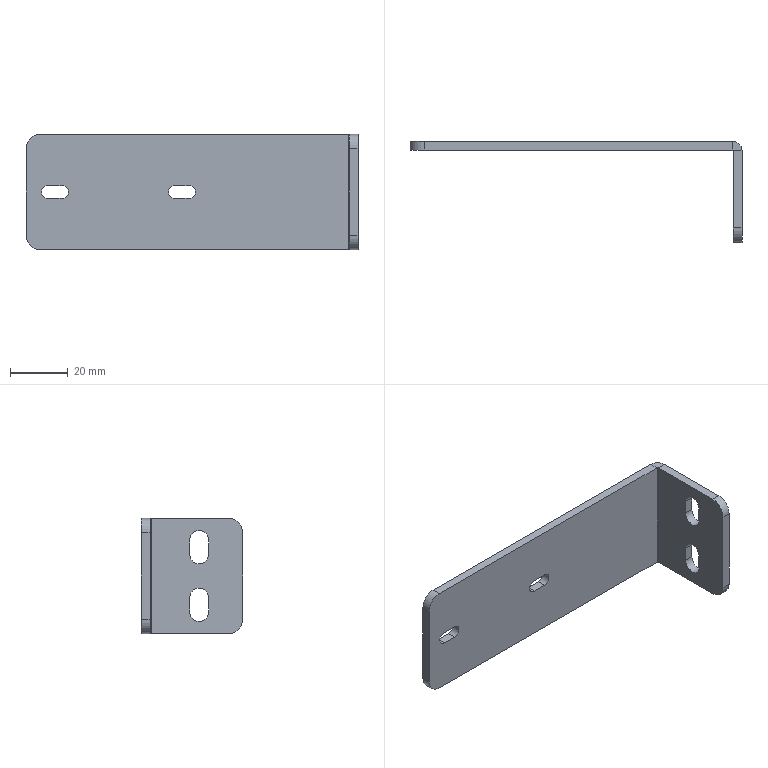Part | SolidWorks | features ICE 2, Fillet 1, FlatPattern 1, HoleWzd 1, SMBaseFlange 1, SheetMetal 1 | 1 solid | 34 faces | box 115 x 35 x 40 mm | volume 16866 mm3 | plane 20 | cylinder 14 | commonest cylinder face diameters 4.4 x4 6.5 x4 10 x4 0.6 x1 6.6 x1
STEP:
#1=CARTESIAN_POINT('',(115.,-3.3,40.));
#2=VERTEX_POINT('',#1);
#3=CARTESIAN_POINT('',(112.,-3.3,40.));
#4=VERTEX_POINT('',#3);
#5=CARTESIAN_POINT('',(115.,-3.3,40.));
#6=DIRECTION('',(-1.,0.,0.));
#7=VECTOR('',#6,1000.);
#8=LINE('',#5,#7);
#9=EDGE_CURVE('',#2,#4,#8,.T.);
#10=ORIENTED_EDGE('',*,*,#9,.F.);
#11=CARTESIAN_POINT('',(111.7,0.,40.));
#12=VERTEX_POINT('',#11);
#13=CARTESIAN_POINT('',(111.7,-3.3,40.));
#14=DIRECTION('',(0.,0.,-1.));
#15=DIRECTION('',(1.,0.,0.));
#16=AXIS2_PLACEMENT_3D('',#13,#14,#15);
#17=CIRCLE('',#16,3.3);
#18=EDGE_CURVE('',#12,#2,#17,.T.);
#19=ORIENTED_EDGE('',*,*,#18,.F.);
#20=CARTESIAN_POINT('',(111.7,-3.,40.));
#21=VERTEX_POINT('',#20);
#22=CARTESIAN_POINT('',(111.7,-3.,40.));
#23=DIRECTION('',(0.,1.,0.));
#24=VECTOR('',#23,1000.);
#25=LINE('',#22,#24);
#26=EDGE_CURVE('',#21,#12,#25,.T.);
#27=ORIENTED_EDGE('',*,*,#26,.F.);
#28=CARTESIAN_POINT('',(111.7,-3.3,40.));
#29=DIRECTION('',(0.,0.,-1.));
#30=DIRECTION('',(1.,0.,0.));
#31=AXIS2_PLACEMENT_3D('',#28,#29,#30);
#32=CIRCLE('',#31,0.3);
#33=EDGE_CURVE('',#21,#4,#32,.T.);
#34=ORIENTED_EDGE('',*,*,#33,.T.);
#35=EDGE_LOOP('',(#10,#19,#27,#34));
#36=FACE_OUTER_BOUND('',#35,.T.);
#37=CARTESIAN_POINT('',(115.,-3.3,40.));
#38=DIRECTION('',(0.,0.,1.));
#39=DIRECTION('',(1.,0.,0.));
#40=AXIS2_PLACEMENT_3D('',#37,#38,#39);
#41=PLANE('',#40);
#42=ADVANCED_FACE('',(#36),#41,.T.);
#43=CARTESIAN_POINT('',(112.,-30.,40.));
#44=VERTEX_POINT('',#43);
#45=CARTESIAN_POINT('',(112.,0.,40.));
#46=DIRECTION('',(0.,-1.,0.));
#47=VECTOR('',#46,1000.);
#48=LINE('',#45,#47);
#49=EDGE_CURVE('',#4,#44,#48,.T.);
#50=ORIENTED_EDGE('',*,*,#49,.T.);
#51=CARTESIAN_POINT('',(115.,-30.,40.));
#52=VERTEX_POINT('',#51);
#53=CARTESIAN_POINT('',(111.7,-30.,40.));
#54=DIRECTION('',(1.,0.,0.));
#55=VECTOR('',#54,1000.);
#56=LINE('',#53,#55);
#57=EDGE_CURVE('',#44,#52,#56,.T.);
#58=ORIENTED_EDGE('',*,*,#57,.T.);
#59=CARTESIAN_POINT('',(115.,0.,40.));
#60=DIRECTION('',(0.,-1.,0.));
#61=VECTOR('',#60,1000.);
#62=LINE('',#59,#61);
#63=EDGE_CURVE('',#2,#52,#62,.T.);
#64=ORIENTED_EDGE('',*,*,#63,.F.);
#65=ORIENTED_EDGE('',*,*,#9,.T.);
#66=EDGE_LOOP('',(#50,#58,#64,#65));
#67=FACE_OUTER_BOUND('',#66,.T.);
#68=CARTESIAN_POINT('',(111.7,-3.,40.));
#69=DIRECTION('',(0.,0.,1.));
#70=DIRECTION('',(1.,0.,0.));
#71=AXIS2_PLACEMENT_3D('',#68,#69,#70);
#72=PLANE('',#71);
#73=ADVANCED_FACE('',(#67),#72,.T.);
#74=CARTESIAN_POINT('',(111.7,0.,0.));
#75=VERTEX_POINT('',#74);
#76=CARTESIAN_POINT('',(111.7,-3.,0.));
#77=VERTEX_POINT('',#76);
#78=CARTESIAN_POINT('',(111.7,0.,0.));
#79=DIRECTION('',(0.,-1.,0.));
#80=VECTOR('',#79,1000.);
#81=LINE('',#78,#80);
#82=EDGE_CURVE('',#75,#77,#81,.T.);
#83=ORIENTED_EDGE('',*,*,#82,.F.);
#84=CARTESIAN_POINT('',(115.,-3.3,0.));
#85=VERTEX_POINT('',#84);
#86=CARTESIAN_POINT('',(111.7,-3.3,0.));
#87=DIRECTION('',(0.,0.,-1.));
#88=DIRECTION('',(1.,0.,0.));
#89=AXIS2_PLACEMENT_3D('',#86,#87,#88);
#90=CIRCLE('',#89,3.3);
#91=EDGE_CURVE('',#75,#85,#90,.T.);
#92=ORIENTED_EDGE('',*,*,#91,.T.);
#93=CARTESIAN_POINT('',(112.,-3.3,0.));
#94=VERTEX_POINT('',#93);
#95=CARTESIAN_POINT('',(112.,-3.3,0.));
#96=DIRECTION('',(1.,0.,0.));
#97=VECTOR('',#96,1000.);
#98=LINE('',#95,#97);
#99=EDGE_CURVE('',#94,#85,#98,.T.);
#100=ORIENTED_EDGE('',*,*,#99,.F.);
#101=CARTESIAN_POINT('',(111.7,-3.3,0.));
#102=DIRECTION('',(0.,0.,-1.));
#103=DIRECTION('',(1.,0.,0.));
#104=AXIS2_PLACEMENT_3D('',#101,#102,#103);
#105=CIRCLE('',#104,0.3);
#106=EDGE_CURVE('',#77,#94,#105,.T.);
#107=ORIENTED_EDGE('',*,*,#106,.F.);
#108=EDGE_LOOP('',(#83,#92,#100,#107));
#109=FACE_OUTER_BOUND('',#108,.T.);
#110=CARTESIAN_POINT('',(111.7,0.,0.));
#111=DIRECTION('',(0.,0.,-1.));
#112=DIRECTION('',(-1.,0.,0.));
#113=AXIS2_PLACEMENT_3D('',#110,#111,#112);
#114=PLANE('',#113);
#115=ADVANCED_FACE('',(#109),#114,.T.);
#116=CARTESIAN_POINT('',(5.,-3.,0.));
#117=VERTEX_POINT('',#116);
#118=CARTESIAN_POINT('',(0.,-3.,0.));
#119=DIRECTION('',(1.,0.,0.));
#120=VECTOR('',#119,1000.);
#121=LINE('',#118,#120);
#122=EDGE_CURVE('',#117,#77,#121,.T.);
#123=ORIENTED_EDGE('',*,*,#122,.F.);
#124=CARTESIAN_POINT('',(5.,0.,0.));
#125=VERTEX_POINT('',#124);
#126=CARTESIAN_POINT('',(5.,-3.3,0.));
#127=DIRECTION('',(0.,1.,0.));
#128=VECTOR('',#127,1000.);
#129=LINE('',#126,#128);
#130=EDGE_CURVE('',#117,#125,#129,.T.);
#131=ORIENTED_EDGE('',*,*,#130,.T.);
#132=CARTESIAN_POINT('',(0.,0.,0.));
#133=DIRECTION('',(1.,0.,0.));
#134=VECTOR('',#133,1000.);
#135=LINE('',#132,#134);
#136=EDGE_CURVE('',#125,#75,#135,.T.);
#137=ORIENTED_EDGE('',*,*,#136,.T.);
#138=ORIENTED_EDGE('',*,*,#82,.T.);
#139=EDGE_LOOP('',(#123,#131,#137,#138));
#140=FACE_OUTER_BOUND('',#139,.T.);
#141=CARTESIAN_POINT('',(112.,-3.3,0.));
#142=DIRECTION('',(0.,0.,-1.));
#143=DIRECTION('',(-1.,0.,0.));
#144=AXIS2_PLACEMENT_3D('',#141,#142,#143);
#145=PLANE('',#144);
#146=ADVANCED_FACE('',(#140),#145,.T.);
#147=CARTESIAN_POINT('',(112.,-23.25,7.5));
#148=VERTEX_POINT('',#147);
#149=CARTESIAN_POINT('',(112.,-23.25,12.5));
#150=VERTEX_POINT('',#149);
#151=CARTESIAN_POINT('',(112.,-23.25,7.5));
#152=DIRECTION('',(0.,0.,1.));
#153=VECTOR('',#152,1000.);
#154=LINE('',#151,#153);
#155=EDGE_CURVE('',#148,#150,#154,.T.);
#156=ORIENTED_EDGE('',*,*,#155,.F.);
#157=CARTESIAN_POINT('',(112.,-16.75,7.5));
#158=VERTEX_POINT('',#157);
#159=CARTESIAN_POINT('',(112.,-20.,7.5));
#160=DIRECTION('',(-1.,0.,0.));
#161=DIRECTION('',(0.,-1.,0.));
#162=AXIS2_PLACEMENT_3D('',#159,#160,#161);
#163=CIRCLE('',#162,3.25);
#164=EDGE_CURVE('',#158,#148,#163,.T.);
#165=ORIENTED_EDGE('',*,*,#164,.F.);
#166=CARTESIAN_POINT('',(112.,-16.75,12.5));
#167=VERTEX_POINT('',#166);
#168=CARTESIAN_POINT('',(112.,-16.75,7.5));
#169=DIRECTION('',(0.,0.,-1.));
#170=VECTOR('',#169,1000.);
#171=LINE('',#168,#170);
#172=EDGE_CURVE('',#167,#158,#171,.T.);
#173=ORIENTED_EDGE('',*,*,#172,.F.);
#174=CARTESIAN_POINT('',(112.,-20.,12.5));
#175=DIRECTION('',(-1.,0.,0.));
#176=DIRECTION('',(0.,-1.,0.));
#177=AXIS2_PLACEMENT_3D('',#174,#175,#176);
#178=CIRCLE('',#177,3.25);
#179=EDGE_CURVE('',#150,#167,#178,.T.);
#180=ORIENTED_EDGE('',*,*,#179,.F.);
#181=EDGE_LOOP('',(#156,#165,#173,#180));
#182=FACE_BOUND('',#181,.T.);
#183=CARTESIAN_POINT('',(112.,-23.25,27.5));
#184=VERTEX_POINT('',#183);
#185=CARTESIAN_POINT('',(112.,-23.25,32.5));
#186=VERTEX_POINT('',#185);
#187=CARTESIAN_POINT('',(112.,-23.25,27.5));
#188=DIRECTION('',(0.,0.,1.));
#189=VECTOR('',#188,1000.);
#190=LINE('',#187,#189);
#191=EDGE_CURVE('',#184,#186,#190,.T.);
#192=ORIENTED_EDGE('',*,*,#191,.F.);
#193=CARTESIAN_POINT('',(112.,-16.75,27.5));
#194=VERTEX_POINT('',#193);
#195=CARTESIAN_POINT('',(112.,-20.,27.5));
#196=DIRECTION('',(-1.,0.,0.));
#197=DIRECTION('',(0.,-1.,0.));
#198=AXIS2_PLACEMENT_3D('',#195,#196,#197);
#199=CIRCLE('',#198,3.25);
#200=EDGE_CURVE('',#194,#184,#199,.T.);
#201=ORIENTED_EDGE('',*,*,#200,.F.);
#202=CARTESIAN_POINT('',(112.,-16.75,32.5));
#203=VERTEX_POINT('',#202);
#204=CARTESIAN_POINT('',(112.,-16.75,27.5));
#205=DIRECTION('',(0.,0.,-1.));
#206=VECTOR('',#205,1000.);
#207=LINE('',#204,#206);
#208=EDGE_CURVE('',#203,#194,#207,.T.);
#209=ORIENTED_EDGE('',*,*,#208,.F.);
#210=CARTESIAN_POINT('',(112.,-20.,32.5));
#211=DIRECTION('',(-1.,0.,0.));
#212=DIRECTION('',(0.,-1.,0.));
#213=AXIS2_PLACEMENT_3D('',#210,#211,#212);
#214=CIRCLE('',#213,3.25);
#215=EDGE_CURVE('',#186,#203,#214,.T.);
#216=ORIENTED_EDGE('',*,*,#215,.F.);
#217=EDGE_LOOP('',(#192,#201,#209,#216));
#218=FACE_BOUND('',#217,.T.);
#219=CARTESIAN_POINT('',(112.,-30.,0.));
#220=VERTEX_POINT('',#219);
#221=CARTESIAN_POINT('',(112.,0.,0.));
#222=DIRECTION('',(0.,-1.,0.));
#223=VECTOR('',#222,1000.);
#224=LINE('',#221,#223);
#225=EDGE_CURVE('',#94,#220,#224,.T.);
#226=ORIENTED_EDGE('',*,*,#225,.T.);
#227=CARTESIAN_POINT('',(112.,-35.,5.));
#228=VERTEX_POINT('',#227);
#229=CARTESIAN_POINT('',(112.,-30.,5.));
#230=DIRECTION('',(-1.,0.,0.));
#231=DIRECTION('',(0.,1.,0.));
#232=AXIS2_PLACEMENT_3D('',#229,#230,#231);
#233=CIRCLE('',#232,5.);
#234=EDGE_CURVE('',#220,#228,#233,.T.);
#235=ORIENTED_EDGE('',*,*,#234,.T.);
#236=CARTESIAN_POINT('',(112.,-35.,35.));
#237=VERTEX_POINT('',#236);
#238=CARTESIAN_POINT('',(112.,-35.,40.));
#239=DIRECTION('',(0.,0.,-1.));
#240=VECTOR('',#239,1000.);
#241=LINE('',#238,#240);
#242=EDGE_CURVE('',#237,#228,#241,.T.);
#243=ORIENTED_EDGE('',*,*,#242,.F.);
#244=CARTESIAN_POINT('',(112.,-30.,35.));
#245=DIRECTION('',(-1.,0.,0.));
#246=DIRECTION('',(0.,1.,0.));
#247=AXIS2_PLACEMENT_3D('',#244,#245,#246);
#248=CIRCLE('',#247,5.);
#249=EDGE_CURVE('',#237,#44,#248,.T.);
#250=ORIENTED_EDGE('',*,*,#249,.T.);
#251=ORIENTED_EDGE('',*,*,#49,.F.);
#252=CARTESIAN_POINT('',(112.,-3.3,40.));
#253=DIRECTION('',(0.,0.,-1.));
#254=VECTOR('',#253,1000.);
#255=LINE('',#252,#254);
#256=EDGE_CURVE('',#4,#94,#255,.T.);
#257=ORIENTED_EDGE('',*,*,#256,.T.);
#258=EDGE_LOOP('',(#226,#235,#243,#250,#251,#257));
#259=FACE_OUTER_BOUND('',#258,.T.);
#260=CARTESIAN_POINT('',(112.,0.,40.));
#261=DIRECTION('',(1.,0.,0.));
#262=DIRECTION('',(0.,1.,0.));
#263=AXIS2_PLACEMENT_3D('',#260,#261,#262);
#264=PLANE('',#263);
#265=ADVANCED_FACE('',(#182,#218,#259),#264,.F.);
#266=ORIENTED_EDGE('',*,*,#242,.T.);
#267=CARTESIAN_POINT('',(115.,-35.,5.));
#268=VERTEX_POINT('',#267);
#269=CARTESIAN_POINT('',(115.,-35.,5.));
#270=DIRECTION('',(1.,0.,0.));
#271=VECTOR('',#270,1000.);
#272=LINE('',#269,#271);
#273=EDGE_CURVE('',#228,#268,#272,.T.);
#274=ORIENTED_EDGE('',*,*,#273,.T.);
#275=CARTESIAN_POINT('',(115.,-35.,35.));
#276=VERTEX_POINT('',#275);
#277=CARTESIAN_POINT('',(115.,-35.,40.));
#278=DIRECTION('',(0.,0.,-1.));
#279=VECTOR('',#278,1000.);
#280=LINE('',#277,#279);
#281=EDGE_CURVE('',#276,#268,#280,.T.);
#282=ORIENTED_EDGE('',*,*,#281,.F.);
#283=CARTESIAN_POINT('',(115.,-35.,35.));
#284=DIRECTION('',(-1.,0.,0.));
#285=VECTOR('',#284,1000.);
#286=LINE('',#283,#285);
#287=EDGE_CURVE('',#276,#237,#286,.T.);
#288=ORIENTED_EDGE('',*,*,#287,.T.);
#289=EDGE_LOOP('',(#266,#274,#282,#288));
#290=FACE_OUTER_BOUND('',#289,.T.);
#291=CARTESIAN_POINT('',(115.,-35.,40.));
#292=DIRECTION('',(0.,-1.,0.));
#293=DIRECTION('',(0.,0.,-1.));
#294=AXIS2_PLACEMENT_3D('',#291,#292,#293);
#295=PLANE('',#294);
#296=ADVANCED_FACE('',(#290),#295,.T.);
#297=CARTESIAN_POINT('',(115.,-23.25,7.5));
#298=VERTEX_POINT('',#297);
#299=CARTESIAN_POINT('',(115.,-16.75,7.5));
#300=VERTEX_POINT('',#299);
#301=CARTESIAN_POINT('',(115.,-20.,7.5));
#302=DIRECTION('',(1.,0.,0.));
#303=DIRECTION('',(0.,1.,0.));
#304=AXIS2_PLACEMENT_3D('',#301,#302,#303);
#305=CIRCLE('',#304,3.25);
#306=EDGE_CURVE('',#298,#300,#305,.T.);
#307=ORIENTED_EDGE('',*,*,#306,.F.);
#308=CARTESIAN_POINT('',(115.,-23.25,12.5));
#309=VERTEX_POINT('',#308);
#310=CARTESIAN_POINT('',(115.,-23.25,40.));
#311=DIRECTION('',(0.,0.,-1.));
#312=VECTOR('',#311,1000.);
#313=LINE('',#310,#312);
#314=EDGE_CURVE('',#309,#298,#313,.T.);
#315=ORIENTED_EDGE('',*,*,#314,.F.);
#316=CARTESIAN_POINT('',(115.,-16.75,12.5));
#317=VERTEX_POINT('',#316);
#318=CARTESIAN_POINT('',(115.,-20.,12.5));
#319=DIRECTION('',(1.,0.,0.));
#320=DIRECTION('',(0.,1.,0.));
#321=AXIS2_PLACEMENT_3D('',#318,#319,#320);
#322=CIRCLE('',#321,3.25);
#323=EDGE_CURVE('',#317,#309,#322,.T.);
#324=ORIENTED_EDGE('',*,*,#323,.F.);
#325=CARTESIAN_POINT('',(115.,-16.75,40.));
#326=DIRECTION('',(0.,0.,1.));
#327=VECTOR('',#326,1000.);
#328=LINE('',#325,#327);
#329=EDGE_CURVE('',#300,#317,#328,.T.);
#330=ORIENTED_EDGE('',*,*,#329,.F.);
#331=EDGE_LOOP('',(#307,#315,#324,#330));
#332=FACE_BOUND('',#331,.T.);
#333=CARTESIAN_POINT('',(115.,-23.25,27.5));
#334=VERTEX_POINT('',#333);
#335=CARTESIAN_POINT('',(115.,-16.75,27.5));
#336=VERTEX_POINT('',#335);
#337=CARTESIAN_POINT('',(115.,-20.,27.5));
#338=DIRECTION('',(1.,0.,0.));
#339=DIRECTION('',(0.,1.,0.));
#340=AXIS2_PLACEMENT_3D('',#337,#338,#339);
#341=CIRCLE('',#340,3.25);
#342=EDGE_CURVE('',#334,#336,#341,.T.);
#343=ORIENTED_EDGE('',*,*,#342,.F.);
#344=CARTESIAN_POINT('',(115.,-23.25,32.5));
#345=VERTEX_POINT('',#344);
#346=CARTESIAN_POINT('',(115.,-23.25,40.));
#347=DIRECTION('',(0.,0.,-1.));
#348=VECTOR('',#347,1000.);
#349=LINE('',#346,#348);
#350=EDGE_CURVE('',#345,#334,#349,.T.);
#351=ORIENTED_EDGE('',*,*,#350,.F.);
#352=CARTESIAN_POINT('',(115.,-16.75,32.5));
#353=VERTEX_POINT('',#352);
#354=CARTESIAN_POINT('',(115.,-20.,32.5));
#355=DIRECTION('',(1.,0.,0.));
#356=DIRECTION('',(0.,1.,0.));
#357=AXIS2_PLACEMENT_3D('',#354,#355,#356);
#358=CIRCLE('',#357,3.25);
#359=EDGE_CURVE('',#353,#345,#358,.T.);
#360=ORIENTED_EDGE('',*,*,#359,.F.);
#361=CARTESIAN_POINT('',(115.,-16.75,40.));
#362=DIRECTION('',(0.,0.,1.));
#363=VECTOR('',#362,1000.);
#364=LINE('',#361,#363);
#365=EDGE_CURVE('',#336,#353,#364,.T.);
#366=ORIENTED_EDGE('',*,*,#365,.F.);
#367=EDGE_LOOP('',(#343,#351,#360,#366));
#368=FACE_BOUND('',#367,.T.);
#369=ORIENTED_EDGE('',*,*,#281,.T.);
#370=CARTESIAN_POINT('',(115.,-30.,0.));
#371=VERTEX_POINT('',#370);
#372=CARTESIAN_POINT('',(115.,-30.,5.));
#373=DIRECTION('',(1.,0.,0.));
#374=DIRECTION('',(0.,1.,0.));
#375=AXIS2_PLACEMENT_3D('',#372,#373,#374);
#376=CIRCLE('',#375,5.);
#377=EDGE_CURVE('',#268,#371,#376,.T.);
#378=ORIENTED_EDGE('',*,*,#377,.T.);
#379=CARTESIAN_POINT('',(115.,0.,0.));
#380=DIRECTION('',(0.,-1.,0.));
#381=VECTOR('',#380,1000.);
#382=LINE('',#379,#381);
#383=EDGE_CURVE('',#85,#371,#382,.T.);
#384=ORIENTED_EDGE('',*,*,#383,.F.);
#385=CARTESIAN_POINT('',(115.,-3.3,40.));
#386=DIRECTION('',(0.,0.,-1.));
#387=VECTOR('',#386,1000.);
#388=LINE('',#385,#387);
#389=EDGE_CURVE('',#2,#85,#388,.T.);
#390=ORIENTED_EDGE('',*,*,#389,.F.);
#391=ORIENTED_EDGE('',*,*,#63,.T.);
#392=CARTESIAN_POINT('',(115.,-30.,35.));
#393=DIRECTION('',(1.,0.,0.));
#394=DIRECTION('',(0.,1.,0.));
#395=AXIS2_PLACEMENT_3D('',#392,#393,#394);
#396=CIRCLE('',#395,5.);
#397=EDGE_CURVE('',#52,#276,#396,.T.);
#398=ORIENTED_EDGE('',*,*,#397,.T.);
#399=EDGE_LOOP('',(#369,#378,#384,#390,#391,#398));
#400=FACE_OUTER_BOUND('',#399,.T.);
#401=CARTESIAN_POINT('',(115.,0.,40.));
#402=DIRECTION('',(1.,0.,0.));
#403=DIRECTION('',(0.,1.,0.));
#404=AXIS2_PLACEMENT_3D('',#401,#402,#403);
#405=PLANE('',#404);
#406=ADVANCED_FACE('',(#332,#368,#400),#405,.T.);
#407=ORIENTED_EDGE('',*,*,#91,.F.);
#408=CARTESIAN_POINT('',(111.7,0.,40.));
#409=DIRECTION('',(0.,0.,-1.));
#410=VECTOR('',#409,1000.);
#411=LINE('',#408,#410);
#412=EDGE_CURVE('',#12,#75,#411,.T.);
#413=ORIENTED_EDGE('',*,*,#412,.F.);
#414=ORIENTED_EDGE('',*,*,#18,.T.);
#415=ORIENTED_EDGE('',*,*,#389,.T.);
#416=EDGE_LOOP('',(#407,#413,#414,#415));
#417=FACE_OUTER_BOUND('',#416,.T.);
#418=CARTESIAN_POINT('',(111.7,-3.3,40.));
#419=DIRECTION('',(0.,0.,-1.));
#420=DIRECTION('',(-1.,0.,0.));
#421=AXIS2_PLACEMENT_3D('',#418,#419,#420);
#422=CYLINDRICAL_SURFACE('',#421,3.3);
#423=ADVANCED_FACE('',(#417),#422,.T.);
#424=CARTESIAN_POINT('',(7.5,0.,17.8));
#425=VERTEX_POINT('',#424);
#426=CARTESIAN_POINT('',(7.5,0.,22.2));
#427=VERTEX_POINT('',#426);
#428=CARTESIAN_POINT('',(7.5,0.,20.));
#429=DIRECTION('',(0.,1.,0.));
#430=DIRECTION('',(0.,0.,1.));
#431=AXIS2_PLACEMENT_3D('',#428,#429,#430);
#432=CIRCLE('',#431,2.2);
#433=EDGE_CURVE('',#425,#427,#432,.T.);
#434=ORIENTED_EDGE('',*,*,#433,.F.);
#435=CARTESIAN_POINT('',(12.5,0.,17.8));
#436=VERTEX_POINT('',#435);
#437=CARTESIAN_POINT('',(0.,0.,17.8));
#438=DIRECTION('',(-1.,0.,0.));
#439=VECTOR('',#438,1000.);
#440=LINE('',#437,#439);
#441=EDGE_CURVE('',#436,#425,#440,.T.);
#442=ORIENTED_EDGE('',*,*,#441,.F.);
#443=CARTESIAN_POINT('',(12.5,0.,22.2));
#444=VERTEX_POINT('',#443);
#445=CARTESIAN_POINT('',(12.5,0.,20.));
#446=DIRECTION('',(0.,1.,0.));
#447=DIRECTION('',(0.,0.,1.));
#448=AXIS2_PLACEMENT_3D('',#445,#446,#447);
#449=CIRCLE('',#448,2.2);
#450=EDGE_CURVE('',#444,#436,#449,.T.);
#451=ORIENTED_EDGE('',*,*,#450,.F.);
#452=CARTESIAN_POINT('',(0.,0.,22.2));
#453=DIRECTION('',(1.,0.,0.));
#454=VECTOR('',#453,1000.);
#455=LINE('',#452,#454);
#456=EDGE_CURVE('',#427,#444,#455,.T.);
#457=ORIENTED_EDGE('',*,*,#456,.F.);
#458=EDGE_LOOP('',(#434,#442,#451,#457));
#459=FACE_BOUND('',#458,.T.);
#460=CARTESIAN_POINT('',(51.5,0.,17.8));
#461=VERTEX_POINT('',#460);
#462=CARTESIAN_POINT('',(51.5,0.,22.2));
#463=VERTEX_POINT('',#462);
#464=CARTESIAN_POINT('',(51.5,0.,20.));
#465=DIRECTION('',(0.,1.,0.));
#466=DIRECTION('',(0.,0.,1.));
#467=AXIS2_PLACEMENT_3D('',#464,#465,#466);
#468=CIRCLE('',#467,2.2);
#469=EDGE_CURVE('',#461,#463,#468,.T.);
#470=ORIENTED_EDGE('',*,*,#469,.F.);
#471=CARTESIAN_POINT('',(56.5,0.,17.8));
#472=VERTEX_POINT('',#471);
#473=CARTESIAN_POINT('',(0.,0.,17.8));
#474=DIRECTION('',(-1.,0.,0.));
#475=VECTOR('',#474,1000.);
#476=LINE('',#473,#475);
#477=EDGE_CURVE('',#472,#461,#476,.T.);
#478=ORIENTED_EDGE('',*,*,#477,.F.);
#479=CARTESIAN_POINT('',(56.5,0.,22.2));
#480=VERTEX_POINT('',#479);
#481=CARTESIAN_POINT('',(56.5,0.,20.));
#482=DIRECTION('',(0.,1.,0.));
#483=DIRECTION('',(0.,0.,1.));
#484=AXIS2_PLACEMENT_3D('',#481,#482,#483);
#485=CIRCLE('',#484,2.2);
#486=EDGE_CURVE('',#480,#472,#485,.T.);
#487=ORIENTED_EDGE('',*,*,#486,.F.);
#488=CARTESIAN_POINT('',(0.,0.,22.2));
#489=DIRECTION('',(1.,0.,0.));
#490=VECTOR('',#489,1000.);
#491=LINE('',#488,#490);
#492=EDGE_CURVE('',#463,#480,#491,.T.);
#493=ORIENTED_EDGE('',*,*,#492,.F.);
#494=EDGE_LOOP('',(#470,#478,#487,#493));
#495=FACE_BOUND('',#494,.T.);
#496=CARTESIAN_POINT('',(0.,0.,35.));
#497=VERTEX_POINT('',#496);
#498=CARTESIAN_POINT('',(0.,0.,5.));
#499=VERTEX_POINT('',#498);
#500=CARTESIAN_POINT('',(0.,0.,40.));
#501=DIRECTION('',(0.,0.,-1.));
#502=VECTOR('',#501,1000.);
#503=LINE('',#500,#502);
#504=EDGE_CURVE('',#497,#499,#503,.T.);
#505=ORIENTED_EDGE('',*,*,#504,.F.);
#506=CARTESIAN_POINT('',(5.,0.,40.));
#507=VERTEX_POINT('',#506);
#508=CARTESIAN_POINT('',(5.,0.,35.));
#509=DIRECTION('',(0.,1.,0.));
#510=DIRECTION('',(0.,0.,1.));
#511=AXIS2_PLACEMENT_3D('',#508,#509,#510);
#512=CIRCLE('',#511,5.);
#513=EDGE_CURVE('',#497,#507,#512,.T.);
#514=ORIENTED_EDGE('',*,*,#513,.T.);
#515=CARTESIAN_POINT('',(0.,0.,40.));
#516=DIRECTION('',(1.,0.,0.));
#517=VECTOR('',#516,1000.);
#518=LINE('',#515,#517);
#519=EDGE_CURVE('',#507,#12,#518,.T.);
#520=ORIENTED_EDGE('',*,*,#519,.T.);
#521=ORIENTED_EDGE('',*,*,#412,.T.);
#522=ORIENTED_EDGE('',*,*,#136,.F.);
#523=CARTESIAN_POINT('',(5.,0.,5.));
#524=DIRECTION('',(0.,1.,0.));
#525=DIRECTION('',(0.,0.,1.));
#526=AXIS2_PLACEMENT_3D('',#523,#524,#525);
#527=CIRCLE('',#526,5.);
#528=EDGE_CURVE('',#125,#499,#527,.T.);
#529=ORIENTED_EDGE('',*,*,#528,.T.);
#530=EDGE_LOOP('',(#505,#514,#520,#521,#522,#529));
#531=FACE_OUTER_BOUND('',#530,.T.);
#532=CARTESIAN_POINT('',(0.,0.,40.));
#533=DIRECTION('',(0.,1.,0.));
#534=DIRECTION('',(0.,0.,1.));
#535=AXIS2_PLACEMENT_3D('',#532,#533,#534);
#536=PLANE('',#535);
#537=ADVANCED_FACE('',(#459,#495,#531),#536,.T.);
#538=CARTESIAN_POINT('',(0.,-3.,35.));
#539=VERTEX_POINT('',#538);
#540=CARTESIAN_POINT('',(0.,-3.,5.));
#541=VERTEX_POINT('',#540);
#542=CARTESIAN_POINT('',(0.,-3.,40.));
#543=DIRECTION('',(0.,0.,-1.));
#544=VECTOR('',#543,1000.);
#545=LINE('',#542,#544);
#546=EDGE_CURVE('',#539,#541,#545,.T.);
#547=ORIENTED_EDGE('',*,*,#546,.F.);
#548=CARTESIAN_POINT('',(0.,-3.,35.));
#549=DIRECTION('',(0.,1.,0.));
#550=VECTOR('',#549,1000.);
#551=LINE('',#548,#550);
#552=EDGE_CURVE('',#539,#497,#551,.T.);
#553=ORIENTED_EDGE('',*,*,#552,.T.);
#554=ORIENTED_EDGE('',*,*,#504,.T.);
#555=CARTESIAN_POINT('',(0.,-3.,5.));
#556=DIRECTION('',(0.,-1.,0.));
#557=VECTOR('',#556,1000.);
#558=LINE('',#555,#557);
#559=EDGE_CURVE('',#499,#541,#558,.T.);
#560=ORIENTED_EDGE('',*,*,#559,.T.);
#561=EDGE_LOOP('',(#547,#553,#554,#560));
#562=FACE_OUTER_BOUND('',#561,.T.);
#563=CARTESIAN_POINT('',(0.,-3.,40.));
#564=DIRECTION('',(-1.,0.,0.));
#565=DIRECTION('',(0.,0.,1.));
#566=AXIS2_PLACEMENT_3D('',#563,#564,#565);
#567=PLANE('',#566);
#568=ADVANCED_FACE('',(#562),#567,.T.);
#569=CARTESIAN_POINT('',(7.5,-3.,17.8));
#570=VERTEX_POINT('',#569);
#571=CARTESIAN_POINT('',(12.5,-3.,17.8));
#572=VERTEX_POINT('',#571);
#573=CARTESIAN_POINT('',(7.5,-3.,17.8));
#574=DIRECTION('',(1.,0.,0.));
#575=VECTOR('',#574,1000.);
#576=LINE('',#573,#575);
#577=EDGE_CURVE('',#570,#572,#576,.T.);
#578=ORIENTED_EDGE('',*,*,#577,.F.);
#579=CARTESIAN_POINT('',(7.5,-3.,22.2));
#580=VERTEX_POINT('',#579);
#581=CARTESIAN_POINT('',(7.5,-3.,20.));
#582=DIRECTION('',(0.,-1.,0.));
#583=DIRECTION('',(0.,0.,-1.));
#584=AXIS2_PLACEMENT_3D('',#581,#582,#583);
#585=CIRCLE('',#584,2.2);
#586=EDGE_CURVE('',#580,#570,#585,.T.);
#587=ORIENTED_EDGE('',*,*,#586,.F.);
#588=CARTESIAN_POINT('',(12.5,-3.,22.2));
#589=VERTEX_POINT('',#588);
#590=CARTESIAN_POINT('',(7.5,-3.,22.2));
#591=DIRECTION('',(-1.,0.,0.));
#592=VECTOR('',#591,1000.);
#593=LINE('',#590,#592);
#594=EDGE_CURVE('',#589,#580,#593,.T.);
#595=ORIENTED_EDGE('',*,*,#594,.F.);
#596=CARTESIAN_POINT('',(12.5,-3.,20.));
#597=DIRECTION('',(0.,-1.,0.));
#598=DIRECTION('',(0.,0.,-1.));
#599=AXIS2_PLACEMENT_3D('',#596,#597,#598);
#600=CIRCLE('',#599,2.2);
#601=EDGE_CURVE('',#572,#589,#600,.T.);
#602=ORIENTED_EDGE('',*,*,#601,.F.);
#603=EDGE_LOOP('',(#578,#587,#595,#602));
#604=FACE_BOUND('',#603,.T.);
#605=CARTESIAN_POINT('',(51.5,-3.,17.8));
#606=VERTEX_POINT('',#605);
#607=CARTESIAN_POINT('',(56.5,-3.,17.8));
#608=VERTEX_POINT('',#607);
#609=CARTESIAN_POINT('',(51.5,-3.,17.8));
#610=DIRECTION('',(1.,0.,0.));
#611=VECTOR('',#610,1000.);
#612=LINE('',#609,#611);
#613=EDGE_CURVE('',#606,#608,#612,.T.);
#614=ORIENTED_EDGE('',*,*,#613,.F.);
#615=CARTESIAN_POINT('',(51.5,-3.,22.2));
#616=VERTEX_POINT('',#615);
#617=CARTESIAN_POINT('',(51.5,-3.,20.));
#618=DIRECTION('',(0.,-1.,0.));
#619=DIRECTION('',(0.,0.,-1.));
#620=AXIS2_PLACEMENT_3D('',#617,#618,#619);
#621=CIRCLE('',#620,2.2);
#622=EDGE_CURVE('',#616,#606,#621,.T.);
#623=ORIENTED_EDGE('',*,*,#622,.F.);
#624=CARTESIAN_POINT('',(56.5,-3.,22.2));
#625=VERTEX_POINT('',#624);
#626=CARTESIAN_POINT('',(51.5,-3.,22.2));
#627=DIRECTION('',(-1.,0.,0.));
#628=VECTOR('',#627,1000.);
#629=LINE('',#626,#628);
#630=EDGE_CURVE('',#625,#616,#629,.T.);
#631=ORIENTED_EDGE('',*,*,#630,.F.);
#632=CARTESIAN_POINT('',(56.5,-3.,20.));
#633=DIRECTION('',(0.,-1.,0.));
#634=DIRECTION('',(0.,0.,-1.));
#635=AXIS2_PLACEMENT_3D('',#632,#633,#634);
#636=CIRCLE('',#635,2.2);
#637=EDGE_CURVE('',#608,#625,#636,.T.);
#638=ORIENTED_EDGE('',*,*,#637,.F.);
#639=EDGE_LOOP('',(#614,#623,#631,#638));
#640=FACE_BOUND('',#639,.T.);
#641=CARTESIAN_POINT('',(5.,-3.,40.));
#642=VERTEX_POINT('',#641);
#643=CARTESIAN_POINT('',(0.,-3.,40.));
#644=DIRECTION('',(1.,0.,0.));
#645=VECTOR('',#644,1000.);
#646=LINE('',#643,#645);
#647=EDGE_CURVE('',#642,#21,#646,.T.);
#648=ORIENTED_EDGE('',*,*,#647,.F.);
#649=CARTESIAN_POINT('',(5.,-3.,35.));
#650=DIRECTION('',(0.,-1.,0.));
#651=DIRECTION('',(0.,0.,1.));
#652=AXIS2_PLACEMENT_3D('',#649,#650,#651);
#653=CIRCLE('',#652,5.);
#654=EDGE_CURVE('',#642,#539,#653,.T.);
#655=ORIENTED_EDGE('',*,*,#654,.T.);
#656=ORIENTED_EDGE('',*,*,#546,.T.);
#657=CARTESIAN_POINT('',(5.,-3.,5.));
#658=DIRECTION('',(0.,-1.,0.));
#659=DIRECTION('',(0.,0.,1.));
#660=AXIS2_PLACEMENT_3D('',#657,#658,#659);
#661=CIRCLE('',#660,5.);
#662=EDGE_CURVE('',#541,#117,#661,.T.);
#663=ORIENTED_EDGE('',*,*,#662,.T.);
#664=ORIENTED_EDGE('',*,*,#122,.T.);
#665=CARTESIAN_POINT('',(111.7,-3.,40.));
#666=DIRECTION('',(0.,0.,-1.));
#667=VECTOR('',#666,1000.);
#668=LINE('',#665,#667);
#669=EDGE_CURVE('',#21,#77,#668,.T.);
#670=ORIENTED_EDGE('',*,*,#669,.F.);
#671=EDGE_LOOP('',(#648,#655,#656,#663,#664,#670));
#672=FACE_OUTER_BOUND('',#671,.T.);
#673=CARTESIAN_POINT('',(0.,-3.,40.));
#674=DIRECTION('',(0.,1.,0.));
#675=DIRECTION('',(0.,0.,1.));
#676=AXIS2_PLACEMENT_3D('',#673,#674,#675);
#677=PLANE('',#676);
#678=ADVANCED_FACE('',(#604,#640,#672),#677,.F.);
#679=ORIENTED_EDGE('',*,*,#106,.T.);
#680=ORIENTED_EDGE('',*,*,#256,.F.);
#681=ORIENTED_EDGE('',*,*,#33,.F.);
#682=ORIENTED_EDGE('',*,*,#669,.T.);
#683=EDGE_LOOP('',(#679,#680,#681,#682));
#684=FACE_OUTER_BOUND('',#683,.T.);
#685=CARTESIAN_POINT('',(111.7,-3.3,40.));
#686=DIRECTION('',(0.,0.,-1.));
#687=DIRECTION('',(-1.,0.,0.));
#688=AXIS2_PLACEMENT_3D('',#685,#686,#687);
#689=CYLINDRICAL_SURFACE('',#688,0.3);
#690=ADVANCED_FACE('',(#684),#689,.F.);
#691=ORIENTED_EDGE('',*,*,#519,.F.);
#692=CARTESIAN_POINT('',(5.,-3.3,40.));
#693=DIRECTION('',(0.,-1.,0.));
#694=VECTOR('',#693,1000.);
#695=LINE('',#692,#694);
#696=EDGE_CURVE('',#507,#642,#695,.T.);
#697=ORIENTED_EDGE('',*,*,#696,.T.);
#698=ORIENTED_EDGE('',*,*,#647,.T.);
#699=ORIENTED_EDGE('',*,*,#26,.T.);
#700=EDGE_LOOP('',(#691,#697,#698,#699));
#701=FACE_OUTER_BOUND('',#700,.T.);
#702=CARTESIAN_POINT('',(111.7,-3.3,40.));
#703=DIRECTION('',(0.,0.,1.));
#704=DIRECTION('',(1.,0.,0.));
#705=AXIS2_PLACEMENT_3D('',#702,#703,#704);
#706=PLANE('',#705);
#707=ADVANCED_FACE('',(#701),#706,.T.);
#708=ORIENTED_EDGE('',*,*,#383,.T.);
#709=CARTESIAN_POINT('',(112.,-30.,0.));
#710=DIRECTION('',(-1.,0.,0.));
#711=VECTOR('',#710,1000.);
#712=LINE('',#709,#711);
#713=EDGE_CURVE('',#371,#220,#712,.T.);
#714=ORIENTED_EDGE('',*,*,#713,.T.);
#715=ORIENTED_EDGE('',*,*,#225,.F.);
#716=ORIENTED_EDGE('',*,*,#99,.T.);
#717=EDGE_LOOP('',(#708,#714,#715,#716));
#718=FACE_OUTER_BOUND('',#717,.T.);
#719=CARTESIAN_POINT('',(111.7,-3.3,0.));
#720=DIRECTION('',(0.,0.,1.));
#721=DIRECTION('',(1.,0.,0.));
#722=AXIS2_PLACEMENT_3D('',#719,#720,#721);
#723=PLANE('',#722);
#724=ADVANCED_FACE('',(#718),#723,.F.);
#725=ORIENTED_EDGE('',*,*,#654,.F.);
#726=ORIENTED_EDGE('',*,*,#696,.F.);
#727=ORIENTED_EDGE('',*,*,#513,.F.);
#728=ORIENTED_EDGE('',*,*,#552,.F.);
#729=EDGE_LOOP('',(#725,#726,#727,#728));
#730=FACE_OUTER_BOUND('',#729,.T.);
#731=CARTESIAN_POINT('',(5.,-3.,35.));
#732=DIRECTION('',(0.,1.,0.));
#733=DIRECTION('',(0.,0.,1.));
#734=AXIS2_PLACEMENT_3D('',#731,#732,#733);
#735=CYLINDRICAL_SURFACE('',#734,5.);
#736=ADVANCED_FACE('',(#730),#735,.T.);
#737=ORIENTED_EDGE('',*,*,#662,.F.);
#738=ORIENTED_EDGE('',*,*,#559,.F.);
#739=ORIENTED_EDGE('',*,*,#528,.F.);
#740=ORIENTED_EDGE('',*,*,#130,.F.);
#741=EDGE_LOOP('',(#737,#738,#739,#740));
#742=FACE_OUTER_BOUND('',#741,.T.);
#743=CARTESIAN_POINT('',(5.,-3.3,5.));
#744=DIRECTION('',(0.,1.,0.));
#745=DIRECTION('',(0.,0.,1.));
#746=AXIS2_PLACEMENT_3D('',#743,#744,#745);
#747=CYLINDRICAL_SURFACE('',#746,5.);
#748=ADVANCED_FACE('',(#742),#747,.T.);
#749=ORIENTED_EDGE('',*,*,#377,.F.);
#750=ORIENTED_EDGE('',*,*,#273,.F.);
#751=ORIENTED_EDGE('',*,*,#234,.F.);
#752=ORIENTED_EDGE('',*,*,#713,.F.);
#753=EDGE_LOOP('',(#749,#750,#751,#752));
#754=FACE_OUTER_BOUND('',#753,.T.);
#755=CARTESIAN_POINT('',(111.7,-30.,5.));
#756=DIRECTION('',(1.,0.,0.));
#757=DIRECTION('',(0.,0.,-1.));
#758=AXIS2_PLACEMENT_3D('',#755,#756,#757);
#759=CYLINDRICAL_SURFACE('',#758,5.);
#760=ADVANCED_FACE('',(#754),#759,.T.);
#761=ORIENTED_EDGE('',*,*,#397,.F.);
#762=ORIENTED_EDGE('',*,*,#57,.F.);
#763=ORIENTED_EDGE('',*,*,#249,.F.);
#764=ORIENTED_EDGE('',*,*,#287,.F.);
#765=EDGE_LOOP('',(#761,#762,#763,#764));
#766=FACE_OUTER_BOUND('',#765,.T.);
#767=CARTESIAN_POINT('',(115.,-30.,35.));
#768=DIRECTION('',(-1.,0.,0.));
#769=DIRECTION('',(0.,0.,1.));
#770=AXIS2_PLACEMENT_3D('',#767,#768,#769);
#771=CYLINDRICAL_SURFACE('',#770,5.);
#772=ADVANCED_FACE('',(#766),#771,.T.);
#773=ORIENTED_EDGE('',*,*,#469,.T.);
#774=CARTESIAN_POINT('',(51.5,7.,22.2));
#775=DIRECTION('',(0.,-1.,0.));
#776=VECTOR('',#775,1000.);
#777=LINE('',#774,#776);
#778=EDGE_CURVE('',#463,#616,#777,.T.);
#779=ORIENTED_EDGE('',*,*,#778,.T.);
#780=ORIENTED_EDGE('',*,*,#622,.T.);
#781=CARTESIAN_POINT('',(51.5,7.,17.8));
#782=DIRECTION('',(0.,-1.,0.));
#783=VECTOR('',#782,1000.);
#784=LINE('',#781,#783);
#785=EDGE_CURVE('',#461,#606,#784,.T.);
#786=ORIENTED_EDGE('',*,*,#785,.F.);
#787=EDGE_LOOP('',(#773,#779,#780,#786));
#788=FACE_OUTER_BOUND('',#787,.T.);
#789=CARTESIAN_POINT('',(51.5,7.,20.));
#790=DIRECTION('',(0.,-1.,0.));
#791=DIRECTION('',(0.,0.,-1.));
#792=AXIS2_PLACEMENT_3D('',#789,#790,#791);
#793=CYLINDRICAL_SURFACE('',#792,2.2);
#794=ADVANCED_FACE('',(#788),#793,.F.);
#795=ORIENTED_EDGE('',*,*,#492,.T.);
#796=CARTESIAN_POINT('',(56.5,7.,22.2));
#797=DIRECTION('',(0.,-1.,0.));
#798=VECTOR('',#797,1000.);
#799=LINE('',#796,#798);
#800=EDGE_CURVE('',#480,#625,#799,.T.);
#801=ORIENTED_EDGE('',*,*,#800,.T.);
#802=ORIENTED_EDGE('',*,*,#630,.T.);
#803=ORIENTED_EDGE('',*,*,#778,.F.);
#804=EDGE_LOOP('',(#795,#801,#802,#803));
#805=FACE_OUTER_BOUND('',#804,.T.);
#806=CARTESIAN_POINT('',(51.5,7.,22.2));
#807=DIRECTION('',(0.,0.,1.));
#808=DIRECTION('',(1.,0.,0.));
#809=AXIS2_PLACEMENT_3D('',#806,#807,#808);
#810=PLANE('',#809);
#811=ADVANCED_FACE('',(#805),#810,.F.);
#812=ORIENTED_EDGE('',*,*,#486,.T.);
#813=CARTESIAN_POINT('',(56.5,7.,17.8));
#814=DIRECTION('',(0.,-1.,0.));
#815=VECTOR('',#814,1000.);
#816=LINE('',#813,#815);
#817=EDGE_CURVE('',#472,#608,#816,.T.);
#818=ORIENTED_EDGE('',*,*,#817,.T.);
#819=ORIENTED_EDGE('',*,*,#637,.T.);
#820=ORIENTED_EDGE('',*,*,#800,.F.);
#821=EDGE_LOOP('',(#812,#818,#819,#820));
#822=FACE_OUTER_BOUND('',#821,.T.);
#823=CARTESIAN_POINT('',(56.5,7.,20.));
#824=DIRECTION('',(0.,-1.,0.));
#825=DIRECTION('',(0.,0.,-1.));
#826=AXIS2_PLACEMENT_3D('',#823,#824,#825);
#827=CYLINDRICAL_SURFACE('',#826,2.2);
#828=ADVANCED_FACE('',(#822),#827,.F.);
#829=ORIENTED_EDGE('',*,*,#477,.T.);
#830=ORIENTED_EDGE('',*,*,#785,.T.);
#831=ORIENTED_EDGE('',*,*,#613,.T.);
#832=ORIENTED_EDGE('',*,*,#817,.F.);
#833=EDGE_LOOP('',(#829,#830,#831,#832));
#834=FACE_OUTER_BOUND('',#833,.T.);
#835=CARTESIAN_POINT('',(51.5,7.,17.8));
#836=DIRECTION('',(0.,0.,-1.));
#837=DIRECTION('',(-1.,0.,0.));
#838=AXIS2_PLACEMENT_3D('',#835,#836,#837);
#839=PLANE('',#838);
#840=ADVANCED_FACE('',(#834),#839,.F.);
#841=ORIENTED_EDGE('',*,*,#433,.T.);
#842=CARTESIAN_POINT('',(7.5,7.,22.2));
#843=DIRECTION('',(0.,-1.,0.));
#844=VECTOR('',#843,1000.);
#845=LINE('',#842,#844);
#846=EDGE_CURVE('',#427,#580,#845,.T.);
#847=ORIENTED_EDGE('',*,*,#846,.T.);
#848=ORIENTED_EDGE('',*,*,#586,.T.);
#849=CARTESIAN_POINT('',(7.5,7.,17.8));
#850=DIRECTION('',(0.,-1.,0.));
#851=VECTOR('',#850,1000.);
#852=LINE('',#849,#851);
#853=EDGE_CURVE('',#425,#570,#852,.T.);
#854=ORIENTED_EDGE('',*,*,#853,.F.);
#855=EDGE_LOOP('',(#841,#847,#848,#854));
#856=FACE_OUTER_BOUND('',#855,.T.);
#857=CARTESIAN_POINT('',(7.5,7.,20.));
#858=DIRECTION('',(0.,-1.,0.));
#859=DIRECTION('',(0.,0.,-1.));
#860=AXIS2_PLACEMENT_3D('',#857,#858,#859);
#861=CYLINDRICAL_SURFACE('',#860,2.2);
#862=ADVANCED_FACE('',(#856),#861,.F.);
#863=ORIENTED_EDGE('',*,*,#456,.T.);
#864=CARTESIAN_POINT('',(12.5,7.,22.2));
#865=DIRECTION('',(0.,-1.,0.));
#866=VECTOR('',#865,1000.);
#867=LINE('',#864,#866);
#868=EDGE_CURVE('',#444,#589,#867,.T.);
#869=ORIENTED_EDGE('',*,*,#868,.T.);
#870=ORIENTED_EDGE('',*,*,#594,.T.);
#871=ORIENTED_EDGE('',*,*,#846,.F.);
#872=EDGE_LOOP('',(#863,#869,#870,#871));
#873=FACE_OUTER_BOUND('',#872,.T.);
#874=CARTESIAN_POINT('',(7.5,7.,22.2));
#875=DIRECTION('',(0.,0.,1.));
#876=DIRECTION('',(1.,0.,0.));
#877=AXIS2_PLACEMENT_3D('',#874,#875,#876);
#878=PLANE('',#877);
#879=ADVANCED_FACE('',(#873),#878,.F.);
#880=ORIENTED_EDGE('',*,*,#450,.T.);
#881=CARTESIAN_POINT('',(12.5,7.,17.8));
#882=DIRECTION('',(0.,-1.,0.));
#883=VECTOR('',#882,1000.);
#884=LINE('',#881,#883);
#885=EDGE_CURVE('',#436,#572,#884,.T.);
#886=ORIENTED_EDGE('',*,*,#885,.T.);
#887=ORIENTED_EDGE('',*,*,#601,.T.);
#888=ORIENTED_EDGE('',*,*,#868,.F.);
#889=EDGE_LOOP('',(#880,#886,#887,#888));
#890=FACE_OUTER_BOUND('',#889,.T.);
#891=CARTESIAN_POINT('',(12.5,7.,20.));
#892=DIRECTION('',(0.,-1.,0.));
#893=DIRECTION('',(0.,0.,-1.));
#894=AXIS2_PLACEMENT_3D('',#891,#892,#893);
#895=CYLINDRICAL_SURFACE('',#894,2.2);
#896=ADVANCED_FACE('',(#890),#895,.F.);
#897=ORIENTED_EDGE('',*,*,#441,.T.);
#898=ORIENTED_EDGE('',*,*,#853,.T.);
#899=ORIENTED_EDGE('',*,*,#577,.T.);
#900=ORIENTED_EDGE('',*,*,#885,.F.);
#901=EDGE_LOOP('',(#897,#898,#899,#900));
#902=FACE_OUTER_BOUND('',#901,.T.);
#903=CARTESIAN_POINT('',(7.5,7.,17.8));
#904=DIRECTION('',(0.,0.,-1.));
#905=DIRECTION('',(-1.,0.,0.));
#906=AXIS2_PLACEMENT_3D('',#903,#904,#905);
#907=PLANE('',#906);
#908=ADVANCED_FACE('',(#902),#907,.F.);
#909=ORIENTED_EDGE('',*,*,#342,.T.);
#910=CARTESIAN_POINT('',(122.,-16.75,27.5));
#911=DIRECTION('',(-1.,0.,0.));
#912=VECTOR('',#911,1000.);
#913=LINE('',#910,#912);
#914=EDGE_CURVE('',#336,#194,#913,.T.);
#915=ORIENTED_EDGE('',*,*,#914,.T.);
#916=ORIENTED_EDGE('',*,*,#200,.T.);
#917=CARTESIAN_POINT('',(122.,-23.25,27.5));
#918=DIRECTION('',(-1.,0.,0.));
#919=VECTOR('',#918,1000.);
#920=LINE('',#917,#919);
#921=EDGE_CURVE('',#334,#184,#920,.T.);
#922=ORIENTED_EDGE('',*,*,#921,.F.);
#923=EDGE_LOOP('',(#909,#915,#916,#922));
#924=FACE_OUTER_BOUND('',#923,.T.);
#925=CARTESIAN_POINT('',(122.,-20.,27.5));
#926=DIRECTION('',(-1.,0.,0.));
#927=DIRECTION('',(0.,-1.,0.));
#928=AXIS2_PLACEMENT_3D('',#925,#926,#927);
#929=CYLINDRICAL_SURFACE('',#928,3.25);
#930=ADVANCED_FACE('',(#924),#929,.F.);
#931=ORIENTED_EDGE('',*,*,#365,.T.);
#932=CARTESIAN_POINT('',(122.,-16.75,32.5));
#933=DIRECTION('',(-1.,0.,0.));
#934=VECTOR('',#933,1000.);
#935=LINE('',#932,#934);
#936=EDGE_CURVE('',#353,#203,#935,.T.);
#937=ORIENTED_EDGE('',*,*,#936,.T.);
#938=ORIENTED_EDGE('',*,*,#208,.T.);
#939=ORIENTED_EDGE('',*,*,#914,.F.);
#940=EDGE_LOOP('',(#931,#937,#938,#939));
#941=FACE_OUTER_BOUND('',#940,.T.);
#942=CARTESIAN_POINT('',(122.,-16.75,27.5));
#943=DIRECTION('',(0.,1.,0.));
#944=DIRECTION('',(-1.,0.,0.));
#945=AXIS2_PLACEMENT_3D('',#942,#943,#944);
#946=PLANE('',#945);
#947=ADVANCED_FACE('',(#941),#946,.F.);
#948=ORIENTED_EDGE('',*,*,#359,.T.);
#949=CARTESIAN_POINT('',(122.,-23.25,32.5));
#950=DIRECTION('',(-1.,0.,0.));
#951=VECTOR('',#950,1000.);
#952=LINE('',#949,#951);
#953=EDGE_CURVE('',#345,#186,#952,.T.);
#954=ORIENTED_EDGE('',*,*,#953,.T.);
#955=ORIENTED_EDGE('',*,*,#215,.T.);
#956=ORIENTED_EDGE('',*,*,#936,.F.);
#957=EDGE_LOOP('',(#948,#954,#955,#956));
#958=FACE_OUTER_BOUND('',#957,.T.);
#959=CARTESIAN_POINT('',(122.,-20.,32.5));
#960=DIRECTION('',(-1.,0.,0.));
#961=DIRECTION('',(0.,-1.,0.));
#962=AXIS2_PLACEMENT_3D('',#959,#960,#961);
#963=CYLINDRICAL_SURFACE('',#962,3.25);
#964=ADVANCED_FACE('',(#958),#963,.F.);
#965=ORIENTED_EDGE('',*,*,#350,.T.);
#966=ORIENTED_EDGE('',*,*,#921,.T.);
#967=ORIENTED_EDGE('',*,*,#191,.T.);
#968=ORIENTED_EDGE('',*,*,#953,.F.);
#969=EDGE_LOOP('',(#965,#966,#967,#968));
#970=FACE_OUTER_BOUND('',#969,.T.);
#971=CARTESIAN_POINT('',(122.,-23.25,27.5));
#972=DIRECTION('',(0.,-1.,0.));
#973=DIRECTION('',(0.,0.,-1.));
#974=AXIS2_PLACEMENT_3D('',#971,#972,#973);
#975=PLANE('',#974);
#976=ADVANCED_FACE('',(#970),#975,.F.);
#977=ORIENTED_EDGE('',*,*,#306,.T.);
#978=CARTESIAN_POINT('',(122.,-16.75,7.5));
#979=DIRECTION('',(-1.,0.,0.));
#980=VECTOR('',#979,1000.);
#981=LINE('',#978,#980);
#982=EDGE_CURVE('',#300,#158,#981,.T.);
#983=ORIENTED_EDGE('',*,*,#982,.T.);
#984=ORIENTED_EDGE('',*,*,#164,.T.);
#985=CARTESIAN_POINT('',(122.,-23.25,7.5));
#986=DIRECTION('',(-1.,0.,0.));
#987=VECTOR('',#986,1000.);
#988=LINE('',#985,#987);
#989=EDGE_CURVE('',#298,#148,#988,.T.);
#990=ORIENTED_EDGE('',*,*,#989,.F.);
#991=EDGE_LOOP('',(#977,#983,#984,#990));
#992=FACE_OUTER_BOUND('',#991,.T.);
#993=CARTESIAN_POINT('',(122.,-20.,7.5));
#994=DIRECTION('',(-1.,0.,0.));
#995=DIRECTION('',(0.,-1.,0.));
#996=AXIS2_PLACEMENT_3D('',#993,#994,#995);
#997=CYLINDRICAL_SURFACE('',#996,3.25);
#998=ADVANCED_FACE('',(#992),#997,.F.);
#999=ORIENTED_EDGE('',*,*,#329,.T.);
#1000=CARTESIAN_POINT('',(122.,-16.75,12.5));
#1001=DIRECTION('',(-1.,0.,0.));
#1002=VECTOR('',#1001,1000.);
#1003=LINE('',#1000,#1002);
#1004=EDGE_CURVE('',#317,#167,#1003,.T.);
#1005=ORIENTED_EDGE('',*,*,#1004,.T.);
#1006=ORIENTED_EDGE('',*,*,#172,.T.);
#1007=ORIENTED_EDGE('',*,*,#982,.F.);
#1008=EDGE_LOOP('',(#999,#1005,#1006,#1007));
#1009=FACE_OUTER_BOUND('',#1008,.T.);
#1010=CARTESIAN_POINT('',(122.,-16.75,7.5));
#1011=DIRECTION('',(0.,1.,0.));
#1012=DIRECTION('',(-1.,0.,0.));
#1013=AXIS2_PLACEMENT_3D('',#1010,#1011,#1012);
#1014=PLANE('',#1013);
#1015=ADVANCED_FACE('',(#1009),#1014,.F.);
#1016=ORIENTED_EDGE('',*,*,#323,.T.);
#1017=CARTESIAN_POINT('',(122.,-23.25,12.5));
#1018=DIRECTION('',(-1.,0.,0.));
#1019=VECTOR('',#1018,1000.);
#1020=LINE('',#1017,#1019);
#1021=EDGE_CURVE('',#309,#150,#1020,.T.);
#1022=ORIENTED_EDGE('',*,*,#1021,.T.);
#1023=ORIENTED_EDGE('',*,*,#179,.T.);
#1024=ORIENTED_EDGE('',*,*,#1004,.F.);
#1025=EDGE_LOOP('',(#1016,#1022,#1023,#1024));
#1026=FACE_OUTER_BOUND('',#1025,.T.);
#1027=CARTESIAN_POINT('',(122.,-20.,12.5));
#1028=DIRECTION('',(-1.,0.,0.));
#1029=DIRECTION('',(0.,-1.,0.));
#1030=AXIS2_PLACEMENT_3D('',#1027,#1028,#1029);
#1031=CYLINDRICAL_SURFACE('',#1030,3.25);
#1032=ADVANCED_FACE('',(#1026),#1031,.F.);
#1033=ORIENTED_EDGE('',*,*,#314,.T.);
#1034=ORIENTED_EDGE('',*,*,#989,.T.);
#1035=ORIENTED_EDGE('',*,*,#155,.T.);
#1036=ORIENTED_EDGE('',*,*,#1021,.F.);
#1037=EDGE_LOOP('',(#1033,#1034,#1035,#1036));
#1038=FACE_OUTER_BOUND('',#1037,.T.);
#1039=CARTESIAN_POINT('',(122.,-23.25,7.5));
#1040=DIRECTION('',(0.,-1.,0.));
#1041=DIRECTION('',(1.,0.,0.));
#1042=AXIS2_PLACEMENT_3D('',#1039,#1040,#1041);
#1043=PLANE('',#1042);
#1044=ADVANCED_FACE('',(#1038),#1043,.F.);
#1045=CLOSED_SHELL('',(#42,#73,#115,#146,#265,#296,#406,#423,#537,#568,#678,#690,#707,#724,#736,#748,#760,#772,#794,#811,#828,#840,#862,#879,#896,#908,#930,#947,#964,#976,#998,#1015,#1032,#1044));
#1046=MANIFOLD_SOLID_BREP('',#1045);
#1047=CARTESIAN_POINT('',(0.,0.,0.));
#1048=DIRECTION('',(0.,0.,1.));
#1049=DIRECTION('',(1.,0.,0.));
#1050=AXIS2_PLACEMENT_3D('',#1047,#1048,#1049);
#1051=(LENGTH_UNIT()NAMED_UNIT(*)SI_UNIT(.MILLI.,.METRE.));
#1052=UNCERTAINTY_MEASURE_WITH_UNIT(LENGTH_MEASURE(0.00001),#1051,'','');
#1053=(NAMED_UNIT(*)PLANE_ANGLE_UNIT()SI_UNIT($,.RADIAN.));
#1054=(NAMED_UNIT(*)SI_UNIT($,.STERADIAN.)SOLID_ANGLE_UNIT());
#1055=(GEOMETRIC_REPRESENTATION_CONTEXT(3)GLOBAL_UNCERTAINTY_ASSIGNED_CONTEXT((#1052))GLOBAL_UNIT_ASSIGNED_CONTEXT((#1051,#1053,#1054))REPRESENTATION_CONTEXT('',''));
#1056=ADVANCED_BREP_SHAPE_REPRESENTATION('',(#1046,#1050),#1055);